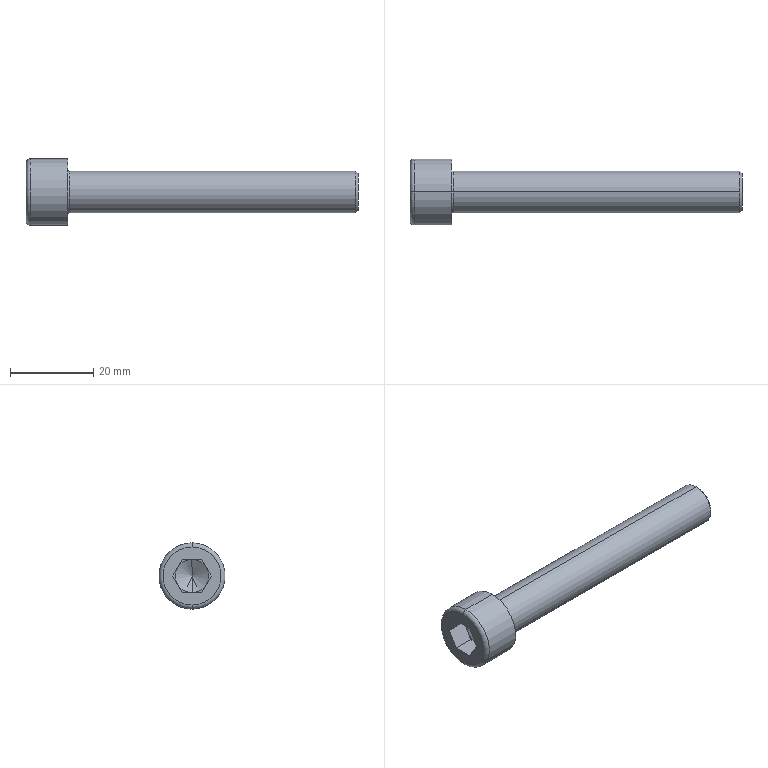Part | STEP file | socket head cap screw fine_din_DIN 912 M10x1 x 70 --- 32N | 1 solid | 27 faces | box 80 x 16 x 16 mm | volume 7176 mm3 | plane 15 | cone 4 | torus 4 | cylinder 4 | commonest cylinder face diameters 10 x2 16 x2